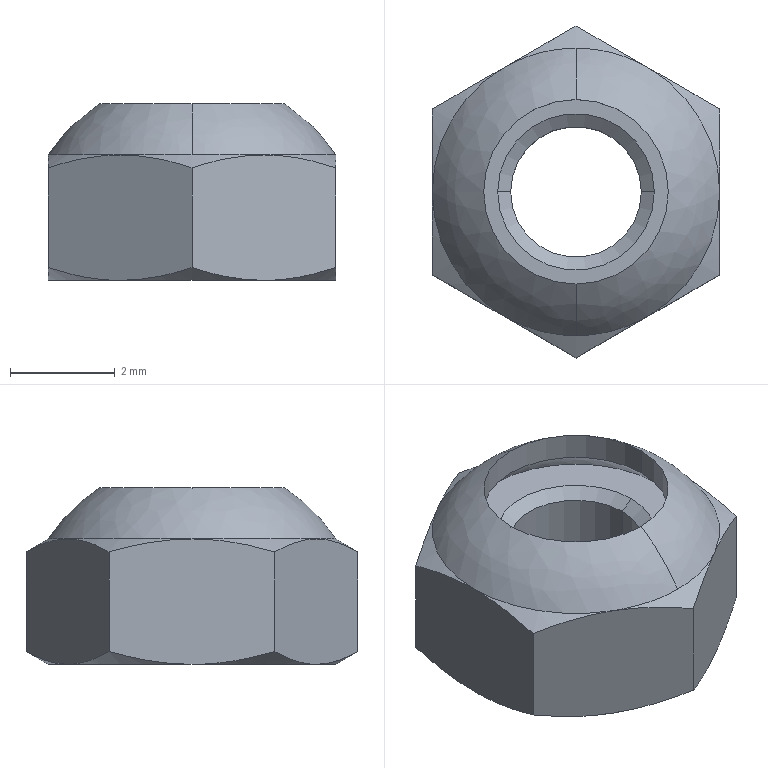Part | STEP file | GB6170-M3 (self-locking)_1 | 1 solid | 34 faces | box 5.5 x 6.351 x 3.382 mm | volume 56.307 mm3 | cone 16 | plane 8 | cylinder 6 | spline 4 | commonest cylinder face diameters 2.5 x2 3 x2 3.532 x2